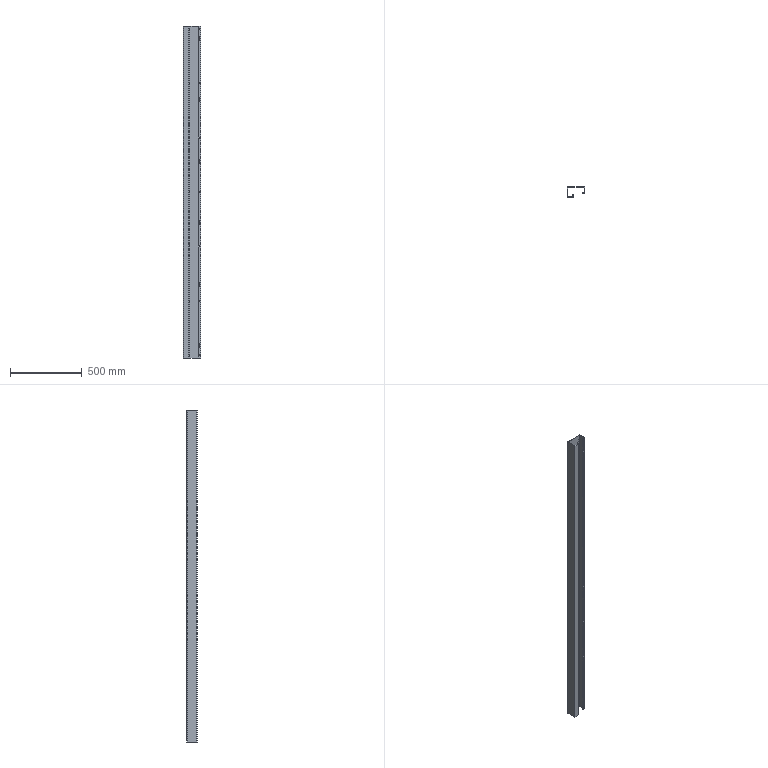Part | 1 solid | 144 faces | box 120 x 70 x 2316 mm | volume 806342 mm3 | plane 80 | cylinder 64 | commonest cylinder face diameters 6.2 x28 9 x18 4 x8 1 x5 3.4 x5